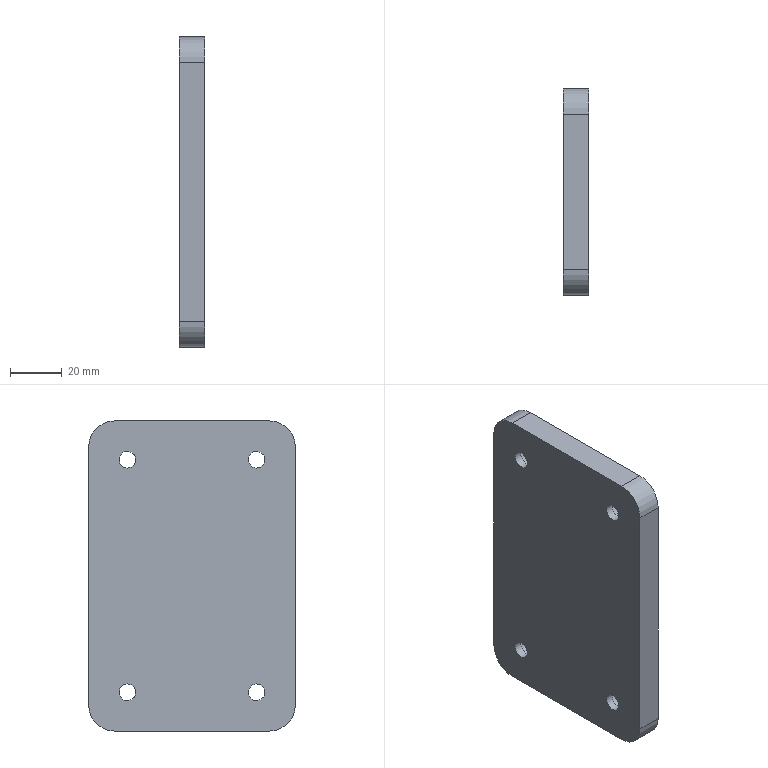Part | STEP file | solid 245 | 1 solid | 22 faces | box 10 x 80 x 120 mm | volume 92082 mm3 | cylinder 12 | plane 10 | commonest cylinder face diameters 6.5 x4 11 x4 20 x4